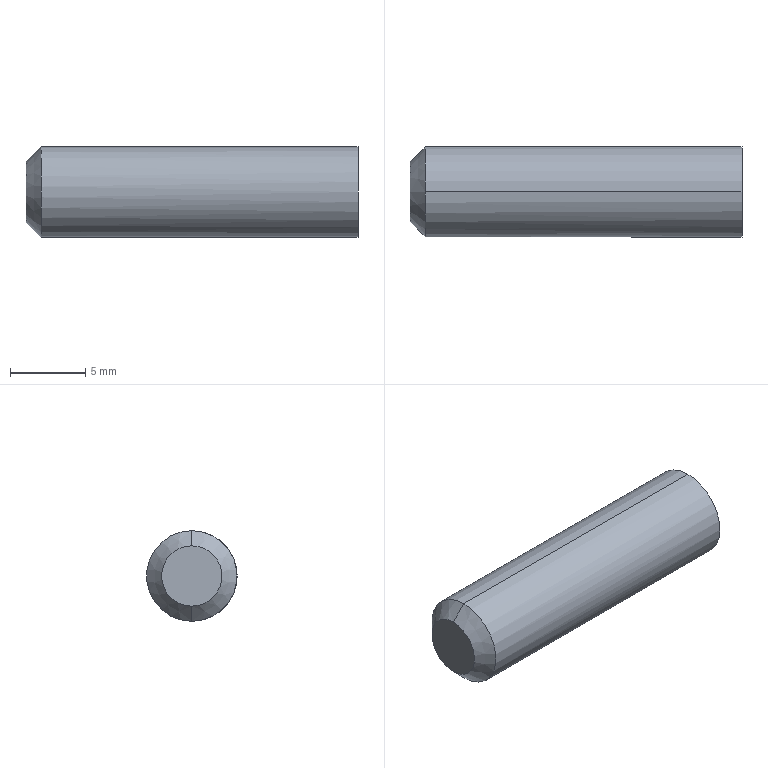Part | STEP file | RJWD-DY-0102_X2_5DE667DC95E8_25 | 1 solid | 6 faces | box 22 x 6 x 6 mm | volume 613.658 mm3 | cylinder 2 | cone 2 | plane 2 | commonest cylinder face diameters 6 x2
STEP:
#1=CARTESIAN_POINT('',(0.,0.,0.));
#2=DIRECTION('',(0.,0.,1.));
#3=DIRECTION('',(1.,0.,0.));
#4=AXIS2_PLACEMENT_3D('',#1,#2,#3);
#5=CARTESIAN_POINT('',(-522.773,4935.973,1684.394));
#6=VERTEX_POINT('',#5);
#7=CARTESIAN_POINT('',(-501.773,4935.973,1684.394));
#8=VERTEX_POINT('',#7);
#9=CARTESIAN_POINT('',(-522.773,4935.973,1684.394));
#10=DIRECTION('',(1.,0.,0.));
#11=VECTOR('',#10,1.);
#12=LINE('',#9,#11);
#13=CARTESIAN_POINT('',(-523.773,4935.973,1681.394));
#14=DIRECTION('',(1.,0.,0.));
#15=DIRECTION('',(0.,0.,-1.));
#16=AXIS2_PLACEMENT_3D('',#13,#14,#15);
#17=CYLINDRICAL_SURFACE('',#16,3.);
#18=CARTESIAN_POINT('',(3.142,1.));
#19=DIRECTION('',(0.,1.));
#20=VECTOR('',#19,1.);
#21=LINE('',#18,#20);
#22=(GEOMETRIC_REPRESENTATION_CONTEXT(2)PARAMETRIC_REPRESENTATION_CONTEXT()REPRESENTATION_CONTEXT('',''));
#23=DEFINITIONAL_REPRESENTATION('',(#21),#22);
#24=PCURVE('',#17,#23);
#25=CARTESIAN_POINT('',(-523.773,4935.973,1681.394));
#26=DIRECTION('',(1.,0.,0.));
#27=DIRECTION('',(0.,0.,-1.));
#28=AXIS2_PLACEMENT_3D('',#25,#26,#27);
#29=CYLINDRICAL_SURFACE('',#28,3.);
#30=CARTESIAN_POINT('',(3.142,1.));
#31=DIRECTION('',(0.,1.));
#32=VECTOR('',#31,1.);
#33=LINE('',#30,#32);
#34=(GEOMETRIC_REPRESENTATION_CONTEXT(2)PARAMETRIC_REPRESENTATION_CONTEXT()REPRESENTATION_CONTEXT('',''));
#35=DEFINITIONAL_REPRESENTATION('',(#33),#34);
#36=PCURVE('',#29,#35);
#37=SURFACE_CURVE('',#12,(#24,#36),.PCURVE_S1.);
#38=EDGE_CURVE('',#6,#8,#37,.T.);
#39=ORIENTED_EDGE('',*,*,#38,.T.);
#40=CARTESIAN_POINT('',(-501.773,4935.973,1678.394));
#41=VERTEX_POINT('',#40);
#42=CARTESIAN_POINT('',(-501.773,4935.973,1681.394));
#43=DIRECTION('',(1.,0.,0.));
#44=DIRECTION('',(0.,0.,-1.));
#45=AXIS2_PLACEMENT_3D('',#42,#43,#44);
#46=CIRCLE('',#45,3.);
#47=CARTESIAN_POINT('',(0.,22.));
#48=DIRECTION('',(1.,0.));
#49=VECTOR('',#48,1.);
#50=LINE('',#47,#49);
#51=(GEOMETRIC_REPRESENTATION_CONTEXT(2)PARAMETRIC_REPRESENTATION_CONTEXT()REPRESENTATION_CONTEXT('',''));
#52=DEFINITIONAL_REPRESENTATION('',(#50),#51);
#53=PCURVE('',#17,#52);
#54=CARTESIAN_POINT('',(-501.773,4935.973,1681.394));
#55=DIRECTION('',(-1.,0.,0.));
#56=DIRECTION('',(0.,0.,1.));
#57=AXIS2_PLACEMENT_3D('',#54,#55,#56);
#58=PLANE('',#57);
#59=CARTESIAN_POINT('',(-3.,0.));
#60=CARTESIAN_POINT('',(-3.,5.196));
#61=CARTESIAN_POINT('',(1.5,2.598));
#62=CARTESIAN_POINT('',(6.,0.));
#63=CARTESIAN_POINT('',(1.5,-2.598));
#64=CARTESIAN_POINT('',(-3.,-5.196));
#65=CARTESIAN_POINT('',(-3.,0.));
#66=(BOUNDED_CURVE()B_SPLINE_CURVE(2,(#59,#60,#61,#62,#63,#64,#65),.UNSPECIFIED.,.T.,.F.)B_SPLINE_CURVE_WITH_KNOTS((1,2,2,2,2,1),(-2.094,0.,2.094,4.189,6.283,8.378),.UNSPECIFIED.)CURVE()GEOMETRIC_REPRESENTATION_ITEM()RATIONAL_B_SPLINE_CURVE((1.,0.5,1.,0.5,1.,0.5,1.))REPRESENTATION_ITEM(''));
#67=(GEOMETRIC_REPRESENTATION_CONTEXT(2)PARAMETRIC_REPRESENTATION_CONTEXT()REPRESENTATION_CONTEXT('',''));
#68=DEFINITIONAL_REPRESENTATION('',(#66),#67);
#69=PCURVE('',#58,#68);
#70=SURFACE_CURVE('',#46,(#53,#69),.PCURVE_S1.);
#71=EDGE_CURVE('',#41,#8,#70,.T.);
#72=ORIENTED_EDGE('',*,*,#71,.F.);
#73=CARTESIAN_POINT('',(-522.773,4935.973,1678.394));
#74=VERTEX_POINT('',#73);
#75=CARTESIAN_POINT('',(-522.773,4935.973,1678.394));
#76=DIRECTION('',(1.,0.,0.));
#77=VECTOR('',#76,1.);
#78=LINE('',#75,#77);
#79=CARTESIAN_POINT('',(0.,1.));
#80=DIRECTION('',(0.,1.));
#81=VECTOR('',#80,1.);
#82=LINE('',#79,#81);
#83=(GEOMETRIC_REPRESENTATION_CONTEXT(2)PARAMETRIC_REPRESENTATION_CONTEXT()REPRESENTATION_CONTEXT('',''));
#84=DEFINITIONAL_REPRESENTATION('',(#82),#83);
#85=PCURVE('',#17,#84);
#86=CARTESIAN_POINT('',(6.283,1.));
#87=DIRECTION('',(0.,1.));
#88=VECTOR('',#87,1.);
#89=LINE('',#86,#88);
#90=(GEOMETRIC_REPRESENTATION_CONTEXT(2)PARAMETRIC_REPRESENTATION_CONTEXT()REPRESENTATION_CONTEXT('',''));
#91=DEFINITIONAL_REPRESENTATION('',(#89),#90);
#92=PCURVE('',#29,#91);
#93=SURFACE_CURVE('',#78,(#85,#92),.PCURVE_S1.);
#94=EDGE_CURVE('',#74,#41,#93,.T.);
#95=ORIENTED_EDGE('',*,*,#94,.F.);
#96=CARTESIAN_POINT('',(-522.773,4935.973,1681.394));
#97=DIRECTION('',(-1.,0.,0.));
#98=DIRECTION('',(0.,0.,1.));
#99=AXIS2_PLACEMENT_3D('',#96,#97,#98);
#100=CIRCLE('',#99,3.);
#101=CARTESIAN_POINT('',(3.142,1.));
#102=DIRECTION('',(-1.,0.));
#103=VECTOR('',#102,1.);
#104=LINE('',#101,#103);
#105=(GEOMETRIC_REPRESENTATION_CONTEXT(2)PARAMETRIC_REPRESENTATION_CONTEXT()REPRESENTATION_CONTEXT('',''));
#106=DEFINITIONAL_REPRESENTATION('',(#104),#105);
#107=PCURVE('',#17,#106);
#108=CARTESIAN_POINT('',(-523.273,4935.973,1681.394));
#109=DIRECTION('',(1.,0.,0.));
#110=DIRECTION('',(0.,0.,-1.));
#111=AXIS2_PLACEMENT_3D('',#108,#109,#110);
#112=CONICAL_SURFACE('',#111,2.5,0.7854);
#113=CARTESIAN_POINT('',(3.142,0.5));
#114=DIRECTION('',(-1.,0.));
#115=VECTOR('',#114,1.);
#116=LINE('',#113,#115);
#117=(GEOMETRIC_REPRESENTATION_CONTEXT(2)PARAMETRIC_REPRESENTATION_CONTEXT()REPRESENTATION_CONTEXT('',''));
#118=DEFINITIONAL_REPRESENTATION('',(#116),#117);
#119=PCURVE('',#112,#118);
#120=SURFACE_CURVE('',#100,(#107,#119),.PCURVE_S1.);
#121=EDGE_CURVE('',#6,#74,#120,.T.);
#122=ORIENTED_EDGE('',*,*,#121,.F.);
#123=EDGE_LOOP('',(#39,#72,#95,#122));
#124=FACE_BOUND('',#123,.T.);
#125=ADVANCED_FACE('',(#124),#17,.T.);
#126=CARTESIAN_POINT('',(-523.773,4935.973,1679.394));
#127=VERTEX_POINT('',#126);
#128=CARTESIAN_POINT('',(-523.773,4935.973,1679.394));
#129=DIRECTION('',(0.7071,0.,-0.7071));
#130=VECTOR('',#129,1.);
#131=LINE('',#128,#130);
#132=CARTESIAN_POINT('',(0.,-0.5));
#133=DIRECTION('',(0.,1.));
#134=VECTOR('',#133,1.);
#135=LINE('',#132,#134);
#136=(GEOMETRIC_REPRESENTATION_CONTEXT(2)PARAMETRIC_REPRESENTATION_CONTEXT()REPRESENTATION_CONTEXT('',''));
#137=DEFINITIONAL_REPRESENTATION('',(#135),#136);
#138=PCURVE('',#112,#137);
#139=CARTESIAN_POINT('',(-523.273,4935.973,1681.394));
#140=DIRECTION('',(1.,0.,0.));
#141=DIRECTION('',(0.,0.,-1.));
#142=AXIS2_PLACEMENT_3D('',#139,#140,#141);
#143=CONICAL_SURFACE('',#142,2.5,0.7854);
#144=CARTESIAN_POINT('',(6.283,-0.5));
#145=DIRECTION('',(0.,1.));
#146=VECTOR('',#145,1.);
#147=LINE('',#144,#146);
#148=(GEOMETRIC_REPRESENTATION_CONTEXT(2)PARAMETRIC_REPRESENTATION_CONTEXT()REPRESENTATION_CONTEXT('',''));
#149=DEFINITIONAL_REPRESENTATION('',(#147),#148);
#150=PCURVE('',#143,#149);
#151=SURFACE_CURVE('',#131,(#138,#150),.PCURVE_S1.);
#152=EDGE_CURVE('',#127,#74,#151,.T.);
#153=ORIENTED_EDGE('',*,*,#152,.F.);
#154=CARTESIAN_POINT('',(-523.773,4935.973,1683.394));
#155=VERTEX_POINT('',#154);
#156=CARTESIAN_POINT('',(-523.773,4935.973,1681.394));
#157=DIRECTION('',(-1.,0.,0.));
#158=DIRECTION('',(0.,0.,1.));
#159=AXIS2_PLACEMENT_3D('',#156,#157,#158);
#160=CIRCLE('',#159,2.);
#161=CARTESIAN_POINT('',(3.142,-0.5));
#162=DIRECTION('',(-1.,0.));
#163=VECTOR('',#162,1.);
#164=LINE('',#161,#163);
#165=(GEOMETRIC_REPRESENTATION_CONTEXT(2)PARAMETRIC_REPRESENTATION_CONTEXT()REPRESENTATION_CONTEXT('',''));
#166=DEFINITIONAL_REPRESENTATION('',(#164),#165);
#167=PCURVE('',#112,#166);
#168=CARTESIAN_POINT('',(-523.773,4935.973,1681.394));
#169=DIRECTION('',(-1.,0.,0.));
#170=DIRECTION('',(0.,0.,1.));
#171=AXIS2_PLACEMENT_3D('',#168,#169,#170);
#172=PLANE('',#171);
#173=CARTESIAN_POINT('',(0.,0.));
#174=DIRECTION('',(1.,0.));
#175=AXIS2_PLACEMENT_2D('',#173,#174);
#176=CIRCLE('',#175,2.);
#177=(GEOMETRIC_REPRESENTATION_CONTEXT(2)PARAMETRIC_REPRESENTATION_CONTEXT()REPRESENTATION_CONTEXT('',''));
#178=DEFINITIONAL_REPRESENTATION('',(#176),#177);
#179=PCURVE('',#172,#178);
#180=SURFACE_CURVE('',#160,(#167,#179),.PCURVE_S1.);
#181=EDGE_CURVE('',#155,#127,#180,.T.);
#182=ORIENTED_EDGE('',*,*,#181,.F.);
#183=CARTESIAN_POINT('',(-523.773,4935.973,1683.394));
#184=DIRECTION('',(0.7071,0.,0.7071));
#185=VECTOR('',#184,1.);
#186=LINE('',#183,#185);
#187=CARTESIAN_POINT('',(3.142,-0.5));
#188=DIRECTION('',(0.,1.));
#189=VECTOR('',#188,1.);
#190=LINE('',#187,#189);
#191=(GEOMETRIC_REPRESENTATION_CONTEXT(2)PARAMETRIC_REPRESENTATION_CONTEXT()REPRESENTATION_CONTEXT('',''));
#192=DEFINITIONAL_REPRESENTATION('',(#190),#191);
#193=PCURVE('',#112,#192);
#194=CARTESIAN_POINT('',(3.142,-0.5));
#195=DIRECTION('',(0.,1.));
#196=VECTOR('',#195,1.);
#197=LINE('',#194,#196);
#198=(GEOMETRIC_REPRESENTATION_CONTEXT(2)PARAMETRIC_REPRESENTATION_CONTEXT()REPRESENTATION_CONTEXT('',''));
#199=DEFINITIONAL_REPRESENTATION('',(#197),#198);
#200=PCURVE('',#143,#199);
#201=SURFACE_CURVE('',#186,(#193,#200),.PCURVE_S1.);
#202=EDGE_CURVE('',#155,#6,#201,.T.);
#203=ORIENTED_EDGE('',*,*,#202,.T.);
#204=ORIENTED_EDGE('',*,*,#121,.T.);
#205=EDGE_LOOP('',(#153,#182,#203,#204));
#206=FACE_BOUND('',#205,.T.);
#207=ADVANCED_FACE('',(#206),#112,.T.);
#208=ORIENTED_EDGE('',*,*,#202,.F.);
#209=CARTESIAN_POINT('',(-523.773,4935.973,1681.394));
#210=DIRECTION('',(-1.,0.,0.));
#211=DIRECTION('',(0.,0.,-1.));
#212=AXIS2_PLACEMENT_3D('',#209,#210,#211);
#213=CIRCLE('',#212,2.);
#214=CARTESIAN_POINT('',(6.283,-0.5));
#215=DIRECTION('',(-1.,0.));
#216=VECTOR('',#215,1.);
#217=LINE('',#214,#216);
#218=(GEOMETRIC_REPRESENTATION_CONTEXT(2)PARAMETRIC_REPRESENTATION_CONTEXT()REPRESENTATION_CONTEXT('',''));
#219=DEFINITIONAL_REPRESENTATION('',(#217),#218);
#220=PCURVE('',#143,#219);
#221=CARTESIAN_POINT('',(0.,0.));
#222=DIRECTION('',(-1.,0.));
#223=AXIS2_PLACEMENT_2D('',#221,#222);
#224=CIRCLE('',#223,2.);
#225=(GEOMETRIC_REPRESENTATION_CONTEXT(2)PARAMETRIC_REPRESENTATION_CONTEXT()REPRESENTATION_CONTEXT('',''));
#226=DEFINITIONAL_REPRESENTATION('',(#224),#225);
#227=PCURVE('',#172,#226);
#228=SURFACE_CURVE('',#213,(#220,#227),.PCURVE_S1.);
#229=EDGE_CURVE('',#127,#155,#228,.T.);
#230=ORIENTED_EDGE('',*,*,#229,.F.);
#231=ORIENTED_EDGE('',*,*,#152,.T.);
#232=CARTESIAN_POINT('',(-522.773,4935.973,1681.394));
#233=DIRECTION('',(-1.,0.,0.));
#234=DIRECTION('',(0.,0.,-1.));
#235=AXIS2_PLACEMENT_3D('',#232,#233,#234);
#236=CIRCLE('',#235,3.);
#237=CARTESIAN_POINT('',(6.283,0.5));
#238=DIRECTION('',(-1.,0.));
#239=VECTOR('',#238,1.);
#240=LINE('',#237,#239);
#241=(GEOMETRIC_REPRESENTATION_CONTEXT(2)PARAMETRIC_REPRESENTATION_CONTEXT()REPRESENTATION_CONTEXT('',''));
#242=DEFINITIONAL_REPRESENTATION('',(#240),#241);
#243=PCURVE('',#143,#242);
#244=CARTESIAN_POINT('',(6.283,1.));
#245=DIRECTION('',(-1.,0.));
#246=VECTOR('',#245,1.);
#247=LINE('',#244,#246);
#248=(GEOMETRIC_REPRESENTATION_CONTEXT(2)PARAMETRIC_REPRESENTATION_CONTEXT()REPRESENTATION_CONTEXT('',''));
#249=DEFINITIONAL_REPRESENTATION('',(#247),#248);
#250=PCURVE('',#29,#249);
#251=SURFACE_CURVE('',#236,(#243,#250),.PCURVE_S1.);
#252=EDGE_CURVE('',#74,#6,#251,.T.);
#253=ORIENTED_EDGE('',*,*,#252,.T.);
#254=EDGE_LOOP('',(#208,#230,#231,#253));
#255=FACE_BOUND('',#254,.T.);
#256=ADVANCED_FACE('',(#255),#143,.T.);
#257=ORIENTED_EDGE('',*,*,#94,.T.);
#258=CARTESIAN_POINT('',(-501.773,4932.973,1681.394));
#259=VERTEX_POINT('',#258);
#260=CARTESIAN_POINT('',(-501.773,4935.973,1681.394));
#261=DIRECTION('',(1.,0.,0.));
#262=DIRECTION('',(0.,-1.,0.));
#263=AXIS2_PLACEMENT_3D('',#260,#261,#262);
#264=CIRCLE('',#263,3.);
#265=CARTESIAN_POINT('',(4.712,22.));
#266=DIRECTION('',(1.,0.));
#267=VECTOR('',#266,1.);
#268=LINE('',#265,#267);
#269=(GEOMETRIC_REPRESENTATION_CONTEXT(2)PARAMETRIC_REPRESENTATION_CONTEXT()REPRESENTATION_CONTEXT('',''));
#270=DEFINITIONAL_REPRESENTATION('',(#268),#269);
#271=PCURVE('',#29,#270);
#272=CARTESIAN_POINT('',(0.,-3.));
#273=CARTESIAN_POINT('',(-5.196,-3.));
#274=CARTESIAN_POINT('',(-2.598,1.5));
#275=CARTESIAN_POINT('',(0.,6.));
#276=CARTESIAN_POINT('',(2.598,1.5));
#277=CARTESIAN_POINT('',(5.196,-3.));
#278=CARTESIAN_POINT('',(0.,-3.));
#279=(BOUNDED_CURVE()B_SPLINE_CURVE(2,(#272,#273,#274,#275,#276,#277,#278),.UNSPECIFIED.,.T.,.F.)B_SPLINE_CURVE_WITH_KNOTS((1,2,2,2,2,1),(-2.094,0.,2.094,4.189,6.283,8.378),.UNSPECIFIED.)CURVE()GEOMETRIC_REPRESENTATION_ITEM()RATIONAL_B_SPLINE_CURVE((1.,0.5,1.,0.5,1.,0.5,1.))REPRESENTATION_ITEM(''));
#280=(GEOMETRIC_REPRESENTATION_CONTEXT(2)PARAMETRIC_REPRESENTATION_CONTEXT()REPRESENTATION_CONTEXT('',''));
#281=DEFINITIONAL_REPRESENTATION('',(#279),#280);
#282=PCURVE('',#58,#281);
#283=SURFACE_CURVE('',#264,(#271,#282),.PCURVE_S1.);
#284=EDGE_CURVE('',#259,#41,#283,.T.);
#285=ORIENTED_EDGE('',*,*,#284,.F.);
#286=CARTESIAN_POINT('',(-501.773,4935.973,1681.394));
#287=DIRECTION('',(1.,0.,0.));
#288=DIRECTION('',(0.,0.,1.));
#289=AXIS2_PLACEMENT_3D('',#286,#287,#288);
#290=CIRCLE('',#289,3.);
#291=CARTESIAN_POINT('',(3.142,22.));
#292=DIRECTION('',(1.,0.));
#293=VECTOR('',#292,1.);
#294=LINE('',#291,#293);
#295=(GEOMETRIC_REPRESENTATION_CONTEXT(2)PARAMETRIC_REPRESENTATION_CONTEXT()REPRESENTATION_CONTEXT('',''));
#296=DEFINITIONAL_REPRESENTATION('',(#294),#295);
#297=PCURVE('',#29,#296);
#298=CARTESIAN_POINT('',(3.,0.));
#299=CARTESIAN_POINT('',(3.,-5.196));
#300=CARTESIAN_POINT('',(-1.5,-2.598));
#301=CARTESIAN_POINT('',(-6.,0.));
#302=CARTESIAN_POINT('',(-1.5,2.598));
#303=CARTESIAN_POINT('',(3.,5.196));
#304=CARTESIAN_POINT('',(3.,0.));
#305=(BOUNDED_CURVE()B_SPLINE_CURVE(2,(#298,#299,#300,#301,#302,#303,#304),.UNSPECIFIED.,.T.,.F.)B_SPLINE_CURVE_WITH_KNOTS((1,2,2,2,2,1),(-2.094,0.,2.094,4.189,6.283,8.378),.UNSPECIFIED.)CURVE()GEOMETRIC_REPRESENTATION_ITEM()RATIONAL_B_SPLINE_CURVE((1.,0.5,1.,0.5,1.,0.5,1.))REPRESENTATION_ITEM(''));
#306=(GEOMETRIC_REPRESENTATION_CONTEXT(2)PARAMETRIC_REPRESENTATION_CONTEXT()REPRESENTATION_CONTEXT('',''));
#307=DEFINITIONAL_REPRESENTATION('',(#305),#306);
#308=PCURVE('',#58,#307);
#309=SURFACE_CURVE('',#290,(#297,#308),.PCURVE_S1.);
#310=EDGE_CURVE('',#8,#259,#309,.T.);
#311=ORIENTED_EDGE('',*,*,#310,.F.);
#312=ORIENTED_EDGE('',*,*,#38,.F.);
#313=ORIENTED_EDGE('',*,*,#252,.F.);
#314=EDGE_LOOP('',(#257,#285,#311,#312,#313));
#315=FACE_BOUND('',#314,.T.);
#316=ADVANCED_FACE('',(#315),#29,.T.);
#317=ORIENTED_EDGE('',*,*,#284,.F.);
#318=ORIENTED_EDGE('',*,*,#310,.F.);
#319=ORIENTED_EDGE('',*,*,#71,.F.);
#320=EDGE_LOOP('',(#317,#318,#319));
#321=FACE_BOUND('',#320,.F.);
#322=ADVANCED_FACE('',(#321),#58,.F.);
#323=ORIENTED_EDGE('',*,*,#181,.F.);
#324=ORIENTED_EDGE('',*,*,#229,.F.);
#325=EDGE_LOOP('',(#323,#324));
#326=FACE_BOUND('',#325,.F.);
#327=ADVANCED_FACE('',(#326),#172,.T.);
#328=CLOSED_SHELL('',(#125,#207,#256,#316,#322,#327));
#329=MANIFOLD_SOLID_BREP('',#328);
#330=(LENGTH_UNIT()NAMED_UNIT(*)SI_UNIT(.MILLI.,.METRE.));
#331=UNCERTAINTY_MEASURE_WITH_UNIT(LENGTH_MEASURE(0.0000001),#330,'','');
#332=(NAMED_UNIT(*)PLANE_ANGLE_UNIT()SI_UNIT($,.RADIAN.));
#333=(NAMED_UNIT(*)SI_UNIT($,.STERADIAN.)SOLID_ANGLE_UNIT());
#334=(GEOMETRIC_REPRESENTATION_CONTEXT(3)GLOBAL_UNCERTAINTY_ASSIGNED_CONTEXT((#331))GLOBAL_UNIT_ASSIGNED_CONTEXT((#330,#332,#333))REPRESENTATION_CONTEXT('',''));
#335=ADVANCED_BREP_SHAPE_REPRESENTATION('',(#4,#329),#334);